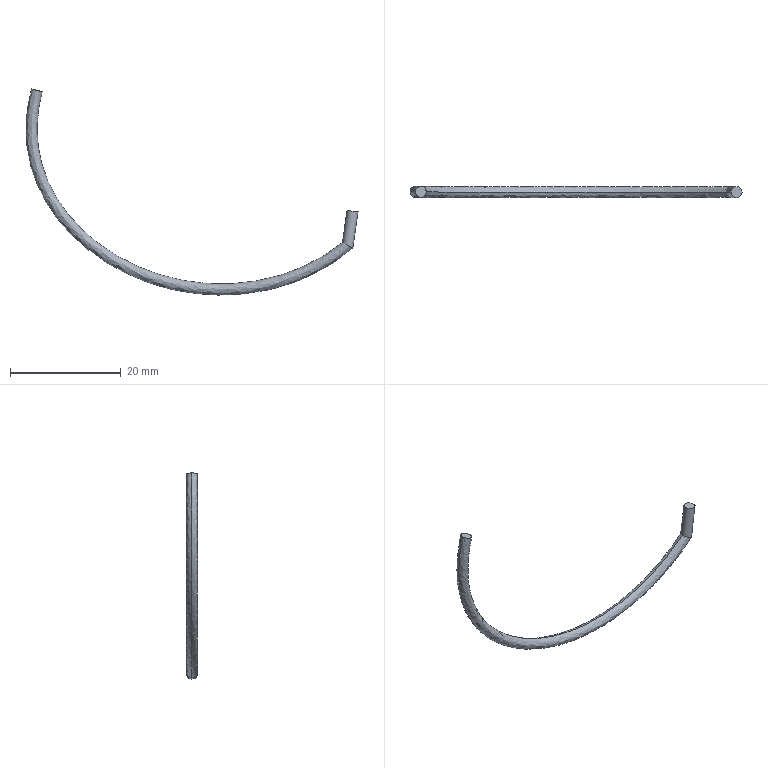Part | STEP file | YINGXIAN2_15_1 | 1 solid | 6 faces | box 59.863 x 2 x 37.179 mm | volume 274.797 mm3 | plane 2 | cylinder 2 | spline 2 | commonest cylinder face diameters 2 x2
STEP:
#1=CARTESIAN_POINT('',(0.,0.,0.));
#2=DIRECTION('',(0.,0.,1.));
#3=DIRECTION('',(1.,0.,0.));
#4=AXIS2_PLACEMENT_3D('',#1,#2,#3);
#5=CARTESIAN_POINT('',(50.419,0.,13.842));
#6=VERTEX_POINT('',#5);
#7=CARTESIAN_POINT('',(52.399,0.,13.558));
#8=VERTEX_POINT('',#7);
#9=CARTESIAN_POINT('',(51.409,0.,13.7));
#10=DIRECTION('',(-0.1418,0.,-0.9899));
#11=DIRECTION('',(-0.9899,0.,0.1418));
#12=AXIS2_PLACEMENT_3D('',#9,#10,#11);
#13=CIRCLE('',#12,1.);
#14=EDGE_CURVE('',#6,#8,#13,.T.);
#15=ORIENTED_EDGE('',*,*,#14,.T.);
#16=CARTESIAN_POINT('',(51.409,0.,13.7));
#17=DIRECTION('',(-0.1418,0.,-0.9899));
#18=DIRECTION('',(0.9899,0.,-0.1418));
#19=AXIS2_PLACEMENT_3D('',#16,#17,#18);
#20=CIRCLE('',#19,1.);
#21=EDGE_CURVE('',#8,#6,#20,.T.);
#22=ORIENTED_EDGE('',*,*,#21,.T.);
#23=EDGE_LOOP('',(#15,#22));
#24=FACE_OUTER_BOUND('',#23,.F.);
#25=CARTESIAN_POINT('',(51.409,0.,13.7));
#26=DIRECTION('',(-0.1418,0.,-0.9899));
#27=DIRECTION('',(-0.9899,0.,0.1418));
#28=AXIS2_PLACEMENT_3D('',#25,#26,#27);
#29=PLANE('',#28);
#30=ADVANCED_FACE('',(#24),#29,.F.);
#31=ORIENTED_EDGE('',*,*,#14,.F.);
#32=CARTESIAN_POINT('',(49.595,0.,8.085));
#33=VERTEX_POINT('',#32);
#34=CARTESIAN_POINT('',(50.419,0.,13.842));
#35=DIRECTION('',(-0.1418,0.,-0.9899));
#36=VECTOR('',#35,5.815);
#37=LINE('',#34,#36);
#38=EDGE_CURVE('',#6,#33,#37,.T.);
#39=ORIENTED_EDGE('',*,*,#38,.T.);
#40=CARTESIAN_POINT('',(50.53,1.,7.56));
#41=VERTEX_POINT('',#40);
#42=CARTESIAN_POINT('',(49.595,0.,8.085));
#43=CARTESIAN_POINT('',(49.595,0.08219,8.085));
#44=CARTESIAN_POINT('',(49.613,0.2494,8.076));
#45=CARTESIAN_POINT('',(49.713,0.5091,8.019));
#46=CARTESIAN_POINT('',(49.85,0.7019,7.942));
#47=CARTESIAN_POINT('',(50.052,0.873,7.828));
#48=CARTESIAN_POINT('',(50.269,0.9721,7.704));
#49=CARTESIAN_POINT('',(50.443,1.,7.611));
#50=B_SPLINE_CURVE_WITH_KNOTS('',3,(#42,#43,#44,#45,#46,#47,#48,#49,#40),.UNSPECIFIED.,.F.,.F.,(4,1,1,1,1,1,4),(0.,0.1667,0.3333,0.5,0.6667,0.8333,1.),.UNSPECIFIED.);
#51=EDGE_CURVE('',#33,#41,#50,.T.);
#52=ORIENTED_EDGE('',*,*,#51,.T.);
#53=CARTESIAN_POINT('',(51.466,0.,7.041));
#54=VERTEX_POINT('',#53);
#55=CARTESIAN_POINT('',(50.53,1.,7.56));
#56=CARTESIAN_POINT('',(50.615,1.,7.51));
#57=CARTESIAN_POINT('',(50.785,0.9732,7.419));
#58=CARTESIAN_POINT('',(50.998,0.8796,7.299));
#59=CARTESIAN_POINT('',(51.21,0.7043,7.182));
#60=CARTESIAN_POINT('',(51.351,0.5023,7.104));
#61=CARTESIAN_POINT('',(51.449,0.2456,7.051));
#62=CARTESIAN_POINT('',(51.466,0.0805,7.041));
#63=B_SPLINE_CURVE_WITH_KNOTS('',3,(#55,#56,#57,#58,#59,#60,#61,#62,#53),.UNSPECIFIED.,.F.,.F.,(4,1,1,1,1,1,4),(0.,0.1667,0.3333,0.5,0.6667,0.8333,1.),.UNSPECIFIED.);
#64=EDGE_CURVE('',#41,#54,#63,.T.);
#65=ORIENTED_EDGE('',*,*,#64,.T.);
#66=CARTESIAN_POINT('',(52.399,0.,13.558));
#67=DIRECTION('',(-0.1418,0.,-0.9899));
#68=VECTOR('',#67,6.584);
#69=LINE('',#66,#68);
#70=EDGE_CURVE('',#8,#54,#69,.T.);
#71=ORIENTED_EDGE('',*,*,#70,.F.);
#72=EDGE_LOOP('',(#31,#39,#52,#65,#71));
#73=FACE_OUTER_BOUND('',#72,.F.);
#74=CARTESIAN_POINT('',(51.409,0.,13.7));
#75=DIRECTION('',(-0.1418,0.,-0.9899));
#76=DIRECTION('',(-0.9899,0.,0.1418));
#77=AXIS2_PLACEMENT_3D('',#74,#75,#76);
#78=CYLINDRICAL_SURFACE('',#77,1.);
#79=ADVANCED_FACE('',(#73),#78,.T.);
#80=ORIENTED_EDGE('',*,*,#21,.F.);
#81=ORIENTED_EDGE('',*,*,#70,.T.);
#82=CARTESIAN_POINT('',(50.53,-1.,7.56));
#83=VERTEX_POINT('',#82);
#84=CARTESIAN_POINT('',(51.466,0.,7.041));
#85=CARTESIAN_POINT('',(51.466,-0.0826,7.041));
#86=CARTESIAN_POINT('',(51.448,-0.2503,7.051));
#87=CARTESIAN_POINT('',(51.348,-0.5086,7.106));
#88=CARTESIAN_POINT('',(51.211,-0.7022,7.182));
#89=CARTESIAN_POINT('',(51.008,-0.8734,7.294));
#90=CARTESIAN_POINT('',(50.79,-0.9723,7.416));
#91=CARTESIAN_POINT('',(50.617,-1.,7.509));
#92=B_SPLINE_CURVE_WITH_KNOTS('',3,(#84,#85,#86,#87,#88,#89,#90,#91,#82),.UNSPECIFIED.,.F.,.F.,(4,1,1,1,1,1,4),(0.,0.1667,0.3333,0.5,0.6667,0.8333,1.),.UNSPECIFIED.);
#93=EDGE_CURVE('',#54,#83,#92,.T.);
#94=ORIENTED_EDGE('',*,*,#93,.T.);
#95=CARTESIAN_POINT('',(50.53,-1.,7.56));
#96=CARTESIAN_POINT('',(50.445,-1.,7.61));
#97=CARTESIAN_POINT('',(50.274,-0.9729,7.702));
#98=CARTESIAN_POINT('',(50.061,-0.879,7.823));
#99=CARTESIAN_POINT('',(49.85,-0.7034,7.942));
#100=CARTESIAN_POINT('',(49.709,-0.5023,8.021));
#101=CARTESIAN_POINT('',(49.612,-0.2439,8.076));
#102=CARTESIAN_POINT('',(49.595,-0.07979,8.085));
#103=CARTESIAN_POINT('',(49.595,0.,8.085));
#104=B_SPLINE_CURVE_WITH_KNOTS('',3,(#95,#96,#97,#98,#99,#100,#101,#102,#103),.UNSPECIFIED.,.F.,.F.,(4,1,1,1,1,1,4),(0.,0.1667,0.3333,0.5,0.6667,0.8333,1.),.UNSPECIFIED.);
#105=EDGE_CURVE('',#83,#33,#104,.T.);
#106=ORIENTED_EDGE('',*,*,#105,.T.);
#107=ORIENTED_EDGE('',*,*,#38,.F.);
#108=EDGE_LOOP('',(#80,#81,#94,#106,#107));
#109=FACE_OUTER_BOUND('',#108,.F.);
#110=CARTESIAN_POINT('',(51.409,0.,13.7));
#111=DIRECTION('',(-0.1418,0.,-0.9899));
#112=DIRECTION('',(-0.9899,0.,0.1418));
#113=AXIS2_PLACEMENT_3D('',#110,#111,#112);
#114=CYLINDRICAL_SURFACE('',#113,1.);
#115=ADVANCED_FACE('',(#109),#114,.T.);
#116=ORIENTED_EDGE('',*,*,#93,.F.);
#117=CARTESIAN_POINT('',(-6.476,0.,35.75));
#118=VERTEX_POINT('',#117);
#119=CARTESIAN_POINT('',(51.466,0.,7.041));
#120=CARTESIAN_POINT('',(51.368,0.,6.957));
#121=CARTESIAN_POINT('',(48.473,0.,4.516));
#122=CARTESIAN_POINT('',(43.598,0.,1.651));
#123=CARTESIAN_POINT('',(36.447,0.,-0.6002));
#124=CARTESIAN_POINT('',(30.891,0.,-1.438));
#125=CARTESIAN_POINT('',(25.282,0.,-1.472));
#126=CARTESIAN_POINT('',(19.88,0.,-0.7714));
#127=CARTESIAN_POINT('',(14.311,0.,0.7748));
#128=CARTESIAN_POINT('',(9.081,0.,3.12));
#129=CARTESIAN_POINT('',(4.225,0.,6.241));
#130=CARTESIAN_POINT('',(-1.55,0.,11.378));
#131=CARTESIAN_POINT('',(-6.039,0.,18.405));
#132=CARTESIAN_POINT('',(-7.838,0.,27.383));
#133=CARTESIAN_POINT('',(-7.264,0.,32.827));
#134=B_SPLINE_CURVE_WITH_KNOTS('',3,(#119,#120,#121,#122,#123,#124,#125,#126,#127,#128,#129,#130,#131,#132,#133,#117),.UNSPECIFIED.,.F.,.F.,(4,1,1,1,1,1,1,1,1,1,1,1,1,4),(0.,0.004598,0.1351,0.2029,0.2764,0.3381,0.4048,0.4716,0.5439,0.6078,0.6771,0.8213,0.9071,1.),.UNSPECIFIED.);
#135=EDGE_CURVE('',#54,#118,#134,.T.);
#136=ORIENTED_EDGE('',*,*,#135,.T.);
#137=CARTESIAN_POINT('',(-4.544,0.,35.23));
#138=VERTEX_POINT('',#137);
#139=CARTESIAN_POINT('',(-4.544,-0.1199,35.23));
#140=CARTESIAN_POINT('',(-4.587,-0.3782,35.241));
#141=CARTESIAN_POINT('',(-4.813,-0.7341,35.302));
#142=CARTESIAN_POINT('',(-5.098,-0.9213,35.379));
#143=CARTESIAN_POINT('',(-5.338,-0.9899,35.444));
#144=CARTESIAN_POINT('',(-5.51,-1.005,35.49));
#145=CARTESIAN_POINT('',(-5.682,-0.9899,35.536));
#146=CARTESIAN_POINT('',(-5.922,-0.9213,35.601));
#147=CARTESIAN_POINT('',(-6.207,-0.7341,35.678));
#148=CARTESIAN_POINT('',(-6.433,-0.3782,35.739));
#149=CARTESIAN_POINT('',(-6.476,-0.1199,35.75));
#150=CARTESIAN_POINT('',(-6.476,0.,35.75));
#151=B_SPLINE_CURVE_WITH_KNOTS('',3,(#137,#139,#140,#141,#142,#143,#144,#145,#146,#147,#148,#149,#150),.UNSPECIFIED.,.F.,.F.,(4,1,1,1,1,1,1,1,1,1,4),(0.,0.125,0.25,0.375,0.4375,0.5,0.5625,0.625,0.75,0.875,1.),.UNSPECIFIED.);
#152=EDGE_CURVE('',#138,#118,#151,.T.);
#153=ORIENTED_EDGE('',*,*,#152,.F.);
#154=CARTESIAN_POINT('',(49.595,0.,8.085));
#155=CARTESIAN_POINT('',(47.029,0.,5.998));
#156=CARTESIAN_POINT('',(42.64,0.,3.449));
#157=CARTESIAN_POINT('',(35.999,0.,1.357));
#158=CARTESIAN_POINT('',(30.732,0.,0.5625));
#159=CARTESIAN_POINT('',(25.408,0.,0.5302));
#160=CARTESIAN_POINT('',(20.278,0.,1.196));
#161=CARTESIAN_POINT('',(14.995,0.,2.662));
#162=CARTESIAN_POINT('',(10.032,0.,4.887));
#163=CARTESIAN_POINT('',(5.436,0.,7.842));
#164=CARTESIAN_POINT('',(0.0008732,0.,12.681));
#165=CARTESIAN_POINT('',(-4.156,0.,19.212));
#166=CARTESIAN_POINT('',(-5.806,0.,27.461));
#167=CARTESIAN_POINT('',(-5.281,0.,32.497));
#168=CARTESIAN_POINT('',(-4.544,0.,35.23));
#169=B_SPLINE_CURVE_WITH_KNOTS('',3,(#154,#155,#156,#157,#158,#159,#160,#161,#162,#163,#164,#165,#166,#167,#168),.UNSPECIFIED.,.F.,.F.,(4,1,1,1,1,1,1,1,1,1,1,1,4),(0.,0.1269,0.1954,0.2696,0.3318,0.3992,0.4666,0.5396,0.6041,0.674,0.8196,0.9062,1.),.UNSPECIFIED.);
#170=EDGE_CURVE('',#33,#138,#169,.T.);
#171=ORIENTED_EDGE('',*,*,#170,.F.);
#172=ORIENTED_EDGE('',*,*,#105,.F.);
#173=EDGE_LOOP('',(#116,#136,#153,#171,#172));
#174=FACE_OUTER_BOUND('',#173,.F.);
#175=CARTESIAN_POINT('',(52.097,0.04715,7.595));
#176=CARTESIAN_POINT('',(51.792,0.04715,7.321));
#177=CARTESIAN_POINT('',(48.712,0.04715,4.658));
#178=CARTESIAN_POINT('',(43.598,0.04715,1.652));
#179=CARTESIAN_POINT('',(36.447,0.04715,-0.5991));
#180=CARTESIAN_POINT('',(30.891,0.04715,-1.437));
#181=CARTESIAN_POINT('',(25.282,0.04715,-1.471));
#182=CARTESIAN_POINT('',(19.88,0.04715,-0.7702));
#183=CARTESIAN_POINT('',(14.312,0.04715,0.7759));
#184=CARTESIAN_POINT('',(9.082,0.04715,3.121));
#185=CARTESIAN_POINT('',(4.225,0.04715,6.242));
#186=CARTESIAN_POINT('',(-1.549,0.04715,11.379));
#187=CARTESIAN_POINT('',(-6.038,0.04715,18.406));
#188=CARTESIAN_POINT('',(-7.884,0.04715,27.621));
#189=CARTESIAN_POINT('',(-7.204,0.04715,33.35));
#190=CARTESIAN_POINT('',(-6.244,0.04715,36.561));
#191=CARTESIAN_POINT('',(52.101,-0.08562,7.59));
#192=CARTESIAN_POINT('',(51.796,-0.08562,7.316));
#193=CARTESIAN_POINT('',(48.715,-0.08562,4.652));
#194=CARTESIAN_POINT('',(43.6,-0.08562,1.646));
#195=CARTESIAN_POINT('',(36.448,-0.08562,-0.6055));
#196=CARTESIAN_POINT('',(30.891,-0.08562,-1.444));
#197=CARTESIAN_POINT('',(25.282,-0.08562,-1.477));
#198=CARTESIAN_POINT('',(19.879,-0.08562,-0.7766));
#199=CARTESIAN_POINT('',(14.309,-0.08562,0.7697));
#200=CARTESIAN_POINT('',(9.078,-0.08562,3.115));
#201=CARTESIAN_POINT('',(4.221,-0.08562,6.237));
#202=CARTESIAN_POINT('',(-1.554,-0.08562,11.375));
#203=CARTESIAN_POINT('',(-6.044,-0.08562,18.403));
#204=CARTESIAN_POINT('',(-7.891,-0.08562,27.621));
#205=CARTESIAN_POINT('',(-7.21,-0.08563,33.351));
#206=CARTESIAN_POINT('',(-6.25,-0.08562,36.563));
#207=CARTESIAN_POINT('',(52.075,-0.3625,7.619));
#208=CARTESIAN_POINT('',(51.77,-0.3625,7.346));
#209=CARTESIAN_POINT('',(48.693,-0.3625,4.685));
#210=CARTESIAN_POINT('',(43.584,-0.3625,1.682));
#211=CARTESIAN_POINT('',(36.439,-0.3625,-0.5669));
#212=CARTESIAN_POINT('',(30.888,-0.3625,-1.404));
#213=CARTESIAN_POINT('',(25.284,-0.3625,-1.438));
#214=CARTESIAN_POINT('',(19.887,-0.3625,-0.7379));
#215=CARTESIAN_POINT('',(14.323,-0.3625,0.8069));
#216=CARTESIAN_POINT('',(9.097,-0.3625,3.15));
#217=CARTESIAN_POINT('',(4.245,-0.3625,6.268));
#218=CARTESIAN_POINT('',(-1.524,-0.3625,11.401));
#219=CARTESIAN_POINT('',(-6.007,-0.3625,18.419));
#220=CARTESIAN_POINT('',(-7.851,-0.3625,27.622));
#221=CARTESIAN_POINT('',(-7.171,-0.3625,33.344));
#222=CARTESIAN_POINT('',(-6.212,-0.3625,36.552));
#223=CARTESIAN_POINT('',(51.912,-0.7341,7.801));
#224=CARTESIAN_POINT('',(51.61,-0.7341,7.529));
#225=CARTESIAN_POINT('',(48.555,-0.7341,4.888));
#226=CARTESIAN_POINT('',(43.482,-0.7341,1.906));
#227=CARTESIAN_POINT('',(36.385,-0.7341,-0.3283));
#228=CARTESIAN_POINT('',(30.869,-0.7341,-1.16));
#229=CARTESIAN_POINT('',(25.3,-0.7341,-1.194));
#230=CARTESIAN_POINT('',(19.935,-0.7341,-0.4981));
#231=CARTESIAN_POINT('',(14.406,-0.7341,1.037));
#232=CARTESIAN_POINT('',(9.213,-0.7341,3.365));
#233=CARTESIAN_POINT('',(4.393,-0.7341,6.464));
#234=CARTESIAN_POINT('',(-1.335,-0.7341,11.559));
#235=CARTESIAN_POINT('',(-5.778,-0.7341,18.517));
#236=CARTESIAN_POINT('',(-7.603,-0.7341,27.629));
#237=CARTESIAN_POINT('',(-6.93,-0.7341,33.299));
#238=CARTESIAN_POINT('',(-5.979,-0.7341,36.482));
#239=CARTESIAN_POINT('',(51.715,-0.9213,8.021));
#240=CARTESIAN_POINT('',(51.415,-0.9213,7.752));
#241=CARTESIAN_POINT('',(48.387,-0.9213,5.134));
#242=CARTESIAN_POINT('',(43.358,-0.9213,2.178));
#243=CARTESIAN_POINT('',(36.318,-0.9213,-0.03895));
#244=CARTESIAN_POINT('',(30.845,-0.9213,-0.8645));
#245=CARTESIAN_POINT('',(25.318,-0.9213,-0.8978));
#246=CARTESIAN_POINT('',(19.994,-0.9213,-0.2073));
#247=CARTESIAN_POINT('',(14.507,-0.9213,1.316));
#248=CARTESIAN_POINT('',(9.354,-0.9213,3.626));
#249=CARTESIAN_POINT('',(4.572,-0.9213,6.7));
#250=CARTESIAN_POINT('',(-1.105,-0.9213,11.752));
#251=CARTESIAN_POINT('',(-5.499,-0.9213,18.637));
#252=CARTESIAN_POINT('',(-7.302,-0.9213,27.638));
#253=CARTESIAN_POINT('',(-6.638,-0.9214,33.244));
#254=CARTESIAN_POINT('',(-5.695,-0.9213,36.397));
#255=CARTESIAN_POINT('',(51.549,-0.9898,8.206));
#256=CARTESIAN_POINT('',(51.251,-0.9898,7.939));
#257=CARTESIAN_POINT('',(48.245,-0.9899,5.34));
#258=CARTESIAN_POINT('',(43.254,-0.9899,2.406));
#259=CARTESIAN_POINT('',(36.262,-0.9899,0.2046));
#260=CARTESIAN_POINT('',(30.825,-0.9899,-0.6155));
#261=CARTESIAN_POINT('',(25.334,-0.9899,-0.6486));
#262=CARTESIAN_POINT('',(20.044,-0.9899,0.03745));
#263=CARTESIAN_POINT('',(14.592,-0.9898,1.551));
#264=CARTESIAN_POINT('',(9.472,-0.9899,3.846));
#265=CARTESIAN_POINT('',(4.723,-0.9899,6.9));
#266=CARTESIAN_POINT('',(-0.9124,-0.9899,11.914));
#267=CARTESIAN_POINT('',(-5.265,-0.9899,18.737));
#268=CARTESIAN_POINT('',(-7.048,-0.9898,27.645));
#269=CARTESIAN_POINT('',(-6.392,-0.9899,33.198));
#270=CARTESIAN_POINT('',(-5.457,-0.9898,36.326));
#271=CARTESIAN_POINT('',(51.43,-1.005,8.338));
#272=CARTESIAN_POINT('',(51.134,-1.005,8.073));
#273=CARTESIAN_POINT('',(48.145,-1.005,5.488));
#274=CARTESIAN_POINT('',(43.179,-1.005,2.569));
#275=CARTESIAN_POINT('',(36.223,-1.005,0.3785));
#276=CARTESIAN_POINT('',(30.811,-1.005,-0.4378));
#277=CARTESIAN_POINT('',(25.345,-1.005,-0.4708));
#278=CARTESIAN_POINT('',(20.079,-1.005,0.2121));
#279=CARTESIAN_POINT('',(14.653,-1.005,1.719));
#280=CARTESIAN_POINT('',(9.557,-1.005,4.003));
#281=CARTESIAN_POINT('',(4.831,-1.005,7.042));
#282=CARTESIAN_POINT('',(-0.7747,-1.005,12.03));
#283=CARTESIAN_POINT('',(-5.097,-1.005,18.809));
#284=CARTESIAN_POINT('',(-6.868,-1.005,27.65));
#285=CARTESIAN_POINT('',(-6.216,-1.005,33.165));
#286=CARTESIAN_POINT('',(-5.287,-1.005,36.275));
#287=CARTESIAN_POINT('',(51.311,-0.9898,8.471));
#288=CARTESIAN_POINT('',(51.017,-0.9898,8.207));
#289=CARTESIAN_POINT('',(48.044,-0.9899,5.636));
#290=CARTESIAN_POINT('',(43.105,-0.9899,2.732));
#291=CARTESIAN_POINT('',(36.183,-0.9899,0.5523));
#292=CARTESIAN_POINT('',(30.797,-0.9899,-0.2602));
#293=CARTESIAN_POINT('',(25.356,-0.9899,-0.293));
#294=CARTESIAN_POINT('',(20.114,-0.9899,0.3868));
#295=CARTESIAN_POINT('',(14.714,-0.9898,1.886));
#296=CARTESIAN_POINT('',(9.641,-0.9899,4.16));
#297=CARTESIAN_POINT('',(4.938,-0.9899,7.184));
#298=CARTESIAN_POINT('',(-0.6369,-0.9899,12.145));
#299=CARTESIAN_POINT('',(-4.93,-0.9899,18.88));
#300=CARTESIAN_POINT('',(-6.687,-0.9898,27.655));
#301=CARTESIAN_POINT('',(-6.041,-0.9899,33.133));
#302=CARTESIAN_POINT('',(-5.117,-0.9898,36.224));
#303=CARTESIAN_POINT('',(51.145,-0.9213,8.656));
#304=CARTESIAN_POINT('',(50.853,-0.9213,8.394));
#305=CARTESIAN_POINT('',(47.903,-0.9213,5.843));
#306=CARTESIAN_POINT('',(43.001,-0.9213,2.961));
#307=CARTESIAN_POINT('',(36.127,-0.9213,0.7959));
#308=CARTESIAN_POINT('',(30.777,-0.9213,-0.0112));
#309=CARTESIAN_POINT('',(25.372,-0.9213,-0.04387));
#310=CARTESIAN_POINT('',(20.164,-0.9213,0.6316));
#311=CARTESIAN_POINT('',(14.799,-0.9213,2.121));
#312=CARTESIAN_POINT('',(9.759,-0.9213,4.38));
#313=CARTESIAN_POINT('',(5.089,-0.9213,7.383));
#314=CARTESIAN_POINT('',(-0.4439,-0.9213,12.307));
#315=CARTESIAN_POINT('',(-4.696,-0.9213,18.981));
#316=CARTESIAN_POINT('',(-6.434,-0.9213,27.663));
#317=CARTESIAN_POINT('',(-5.795,-0.9214,33.087));
#318=CARTESIAN_POINT('',(-4.878,-0.9213,36.153));
#319=CARTESIAN_POINT('',(50.948,-0.7341,8.876));
#320=CARTESIAN_POINT('',(50.658,-0.7341,8.616));
#321=CARTESIAN_POINT('',(47.735,-0.7341,6.088));
#322=CARTESIAN_POINT('',(42.877,-0.7341,3.232));
#323=CARTESIAN_POINT('',(36.061,-0.7341,1.085));
#324=CARTESIAN_POINT('',(30.754,-0.7341,0.2845));
#325=CARTESIAN_POINT('',(25.39,-0.7341,0.2521));
#326=CARTESIAN_POINT('',(20.222,-0.7341,0.9224));
#327=CARTESIAN_POINT('',(14.9,-0.7341,2.4));
#328=CARTESIAN_POINT('',(9.9,-0.7341,4.642));
#329=CARTESIAN_POINT('',(5.268,-0.7341,7.62));
#330=CARTESIAN_POINT('',(-0.2146,-0.7341,12.5));
#331=CARTESIAN_POINT('',(-4.417,-0.7341,19.1));
#332=CARTESIAN_POINT('',(-6.133,-0.7341,27.671));
#333=CARTESIAN_POINT('',(-5.502,-0.7341,33.032));
#334=CARTESIAN_POINT('',(-4.595,-0.7341,36.068));
#335=CARTESIAN_POINT('',(50.785,-0.3629,9.057));
#336=CARTESIAN_POINT('',(50.498,-0.3629,8.8));
#337=CARTESIAN_POINT('',(47.597,-0.3629,6.291));
#338=CARTESIAN_POINT('',(42.775,-0.3629,3.455));
#339=CARTESIAN_POINT('',(36.006,-0.3629,1.324));
#340=CARTESIAN_POINT('',(30.734,-0.3629,0.5282));
#341=CARTESIAN_POINT('',(25.406,-0.3629,0.4959));
#342=CARTESIAN_POINT('',(20.271,-0.3629,1.162));
#343=CARTESIAN_POINT('',(14.983,-0.3629,2.63));
#344=CARTESIAN_POINT('',(10.016,-0.3629,4.857));
#345=CARTESIAN_POINT('',(5.416,-0.3629,7.815));
#346=CARTESIAN_POINT('',(-0.02568,-0.3629,12.659));
#347=CARTESIAN_POINT('',(-4.188,-0.3629,19.198));
#348=CARTESIAN_POINT('',(-5.885,-0.3629,27.678));
#349=CARTESIAN_POINT('',(-5.261,-0.3629,32.987));
#350=CARTESIAN_POINT('',(-4.362,-0.3629,35.998));
#351=CARTESIAN_POINT('',(50.759,-0.08642,9.087));
#352=CARTESIAN_POINT('',(50.472,-0.08642,8.829));
#353=CARTESIAN_POINT('',(47.574,-0.08642,6.324));
#354=CARTESIAN_POINT('',(42.758,-0.08642,3.492));
#355=CARTESIAN_POINT('',(35.997,-0.08642,1.362));
#356=CARTESIAN_POINT('',(30.731,-0.08642,0.5677));
#357=CARTESIAN_POINT('',(25.408,-0.08642,0.5355));
#358=CARTESIAN_POINT('',(20.279,-0.08642,1.201));
#359=CARTESIAN_POINT('',(14.996,-0.08642,2.667));
#360=CARTESIAN_POINT('',(10.035,-0.08642,4.892));
#361=CARTESIAN_POINT('',(5.44,-0.08642,7.847));
#362=CARTESIAN_POINT('',(0.004959,-0.08642,12.684));
#363=CARTESIAN_POINT('',(-4.151,-0.08642,19.214));
#364=CARTESIAN_POINT('',(-5.845,-0.08642,27.68));
#365=CARTESIAN_POINT('',(-5.222,-0.08643,32.98));
#366=CARTESIAN_POINT('',(-4.324,-0.08642,35.987));
#367=CARTESIAN_POINT('',(50.763,0.04607,9.082));
#368=CARTESIAN_POINT('',(50.476,0.04607,8.825));
#369=CARTESIAN_POINT('',(47.578,0.04607,6.319));
#370=CARTESIAN_POINT('',(42.761,0.04607,3.486));
#371=CARTESIAN_POINT('',(35.999,0.04607,1.356));
#372=CARTESIAN_POINT('',(30.732,0.04607,0.5614));
#373=CARTESIAN_POINT('',(25.408,0.04607,0.5291));
#374=CARTESIAN_POINT('',(20.277,0.04607,1.195));
#375=CARTESIAN_POINT('',(14.994,0.04607,2.661));
#376=CARTESIAN_POINT('',(10.032,0.04607,4.886));
#377=CARTESIAN_POINT('',(5.436,0.04607,7.841));
#378=CARTESIAN_POINT('',(0.00001944,0.04607,12.68));
#379=CARTESIAN_POINT('',(-4.157,0.04607,19.212));
#380=CARTESIAN_POINT('',(-5.851,0.04606,27.679));
#381=CARTESIAN_POINT('',(-5.229,0.04607,32.981));
#382=CARTESIAN_POINT('',(-4.33,0.04607,35.989));
#383=B_SPLINE_SURFACE_WITH_KNOTS('',3,3,((#175,#176,#177,#178,#179,#180,#181,#182,#183,#184,#185,#186,#187,#188,#189,#190),(#191,#192,#193,#194,#195,#196,#197,#198,#199,#200,#201,#202,#203,#204,#205,#206),(#207,#208,#209,#210,#211,#212,#213,#214,#215,#216,#217,#218,#219,#220,#221,#222),(#223,#224,#225,#226,#227,#228,#229,#230,#231,#232,#233,#234,#235,#236,#237,#238),(#239,#240,#241,#242,#243,#244,#245,#246,#247,#248,#249,#250,#251,#252,#253,#254),(#255,#256,#257,#258,#259,#260,#261,#262,#263,#264,#265,#266,#267,#268,#269,#270),(#271,#272,#273,#274,#275,#276,#277,#278,#279,#280,#281,#282,#283,#284,#285,#286),(#287,#288,#289,#290,#291,#292,#293,#294,#295,#296,#297,#298,#299,#300,#301,#302),(#303,#304,#305,#306,#307,#308,#309,#310,#311,#312,#313,#314,#315,#316,#317,#318),(#319,#320,#321,#322,#323,#324,#325,#326,#327,#328,#329,#330,#331,#332,#333,#334),(#335,#336,#337,#338,#339,#340,#341,#342,#343,#344,#345,#346,#347,#348,#349,#350),(#351,#352,#353,#354,#355,#356,#357,#358,#359,#360,#361,#362,#363,#364,#365,#366),(#367,#368,#369,#370,#371,#372,#373,#374,#375,#376,#377,#378,#379,#380,#381,#382)),.UNSPECIFIED.,.F.,.F.,.F.,(4,1,1,1,1,1,1,1,1,1,4),(4,1,1,1,1,1,1,1,1,1,1,1,1,4),(0.02517,0.2923,0.5282,0.7641,0.8821,1.,1.118,1.236,1.472,1.708,1.974),(-0.01463,0.,0.1311,0.1993,0.2731,0.335,0.4021,0.4692,0.5418,0.606,0.6756,0.8204,0.9066,1.009),.UNSPECIFIED.);
#384=ADVANCED_FACE('',(#174),#383,.T.);
#385=ORIENTED_EDGE('',*,*,#51,.F.);
#386=ORIENTED_EDGE('',*,*,#170,.T.);
#387=CARTESIAN_POINT('',(-6.476,0.,35.75));
#388=CARTESIAN_POINT('',(-6.476,0.1199,35.75));
#389=CARTESIAN_POINT('',(-6.433,0.3782,35.739));
#390=CARTESIAN_POINT('',(-6.207,0.7341,35.678));
#391=CARTESIAN_POINT('',(-5.922,0.9213,35.601));
#392=CARTESIAN_POINT('',(-5.682,0.9899,35.536));
#393=CARTESIAN_POINT('',(-5.51,1.005,35.49));
#394=CARTESIAN_POINT('',(-5.338,0.9899,35.444));
#395=CARTESIAN_POINT('',(-5.098,0.9213,35.379));
#396=CARTESIAN_POINT('',(-4.813,0.7341,35.302));
#397=CARTESIAN_POINT('',(-4.587,0.3782,35.241));
#398=CARTESIAN_POINT('',(-4.544,0.1199,35.23));
#399=CARTESIAN_POINT('',(-4.544,0.,35.23));
#400=B_SPLINE_CURVE_WITH_KNOTS('',3,(#387,#388,#389,#390,#391,#392,#393,#394,#395,#396,#397,#398,#399),.UNSPECIFIED.,.F.,.F.,(4,1,1,1,1,1,1,1,1,1,4),(0.,0.125,0.25,0.375,0.4375,0.5,0.5625,0.625,0.75,0.875,1.),.UNSPECIFIED.);
#401=EDGE_CURVE('',#118,#138,#400,.T.);
#402=ORIENTED_EDGE('',*,*,#401,.F.);
#403=ORIENTED_EDGE('',*,*,#135,.F.);
#404=ORIENTED_EDGE('',*,*,#64,.F.);
#405=EDGE_LOOP('',(#385,#386,#402,#403,#404));
#406=FACE_OUTER_BOUND('',#405,.F.);
#407=CARTESIAN_POINT('',(50.763,-0.04715,9.082));
#408=CARTESIAN_POINT('',(50.476,-0.04715,8.825));
#409=CARTESIAN_POINT('',(47.578,-0.04715,6.318));
#410=CARTESIAN_POINT('',(42.761,-0.04715,3.486));
#411=CARTESIAN_POINT('',(35.999,-0.04715,1.356));
#412=CARTESIAN_POINT('',(30.732,-0.04715,0.5613));
#413=CARTESIAN_POINT('',(25.408,-0.04715,0.5291));
#414=CARTESIAN_POINT('',(20.277,-0.04715,1.195));
#415=CARTESIAN_POINT('',(14.994,-0.04715,2.661));
#416=CARTESIAN_POINT('',(10.032,-0.04715,4.886));
#417=CARTESIAN_POINT('',(5.436,-0.04715,7.841));
#418=CARTESIAN_POINT('',(-0.0000215,-0.04715,12.68));
#419=CARTESIAN_POINT('',(-4.157,-0.04715,19.212));
#420=CARTESIAN_POINT('',(-5.851,-0.04715,27.679));
#421=CARTESIAN_POINT('',(-5.229,-0.04715,32.981));
#422=CARTESIAN_POINT('',(-4.33,-0.04715,35.989));
#423=CARTESIAN_POINT('',(50.759,0.08562,9.087));
#424=CARTESIAN_POINT('',(50.472,0.08562,8.829));
#425=CARTESIAN_POINT('',(47.574,0.08562,6.324));
#426=CARTESIAN_POINT('',(42.758,0.08562,3.492));
#427=CARTESIAN_POINT('',(35.997,0.08562,1.362));
#428=CARTESIAN_POINT('',(30.731,0.08562,0.5678));
#429=CARTESIAN_POINT('',(25.408,0.08562,0.5356));
#430=CARTESIAN_POINT('',(20.279,0.08562,1.201));
#431=CARTESIAN_POINT('',(14.997,0.08562,2.667));
#432=CARTESIAN_POINT('',(10.035,0.08562,4.892));
#433=CARTESIAN_POINT('',(5.44,0.08562,7.847));
#434=CARTESIAN_POINT('',(0.005048,0.08562,12.685));
#435=CARTESIAN_POINT('',(-4.15,0.08562,19.214));
#436=CARTESIAN_POINT('',(-5.845,0.08562,27.68));
#437=CARTESIAN_POINT('',(-5.222,0.08563,32.98));
#438=CARTESIAN_POINT('',(-4.324,0.08562,35.987));
#439=CARTESIAN_POINT('',(50.785,0.3625,9.057));
#440=CARTESIAN_POINT('',(50.498,0.3625,8.8));
#441=CARTESIAN_POINT('',(47.596,0.3625,6.291));
#442=CARTESIAN_POINT('',(42.775,0.3625,3.456));
#443=CARTESIAN_POINT('',(36.006,0.3625,1.324));
#444=CARTESIAN_POINT('',(30.734,0.3625,0.5284));
#445=CARTESIAN_POINT('',(25.406,0.3625,0.4962));
#446=CARTESIAN_POINT('',(20.271,0.3625,1.162));
#447=CARTESIAN_POINT('',(14.983,0.3625,2.63));
#448=CARTESIAN_POINT('',(10.016,0.3625,4.857));
#449=CARTESIAN_POINT('',(5.416,0.3625,7.815));
#450=CARTESIAN_POINT('',(-0.0255,0.3625,12.659));
#451=CARTESIAN_POINT('',(-4.188,0.3625,19.198));
#452=CARTESIAN_POINT('',(-5.885,0.3625,27.678));
#453=CARTESIAN_POINT('',(-5.261,0.3625,32.987));
#454=CARTESIAN_POINT('',(-4.361,0.3625,35.998));
#455=CARTESIAN_POINT('',(50.948,0.7341,8.876));
#456=CARTESIAN_POINT('',(50.658,0.7341,8.616));
#457=CARTESIAN_POINT('',(47.735,0.7341,6.088));
#458=CARTESIAN_POINT('',(42.877,0.7341,3.232));
#459=CARTESIAN_POINT('',(36.061,0.7341,1.085));
#460=CARTESIAN_POINT('',(30.754,0.7341,0.2845));
#461=CARTESIAN_POINT('',(25.39,0.7341,0.2521));
#462=CARTESIAN_POINT('',(20.222,0.7341,0.9224));
#463=CARTESIAN_POINT('',(14.9,0.7341,2.4));
#464=CARTESIAN_POINT('',(9.9,0.7341,4.642));
#465=CARTESIAN_POINT('',(5.268,0.7341,7.62));
#466=CARTESIAN_POINT('',(-0.2146,0.7341,12.5));
#467=CARTESIAN_POINT('',(-4.417,0.7341,19.1));
#468=CARTESIAN_POINT('',(-6.133,0.7341,27.671));
#469=CARTESIAN_POINT('',(-5.502,0.7341,33.032));
#470=CARTESIAN_POINT('',(-4.595,0.7341,36.068));
#471=CARTESIAN_POINT('',(51.145,0.9213,8.656));
#472=CARTESIAN_POINT('',(50.853,0.9213,8.394));
#473=CARTESIAN_POINT('',(47.903,0.9213,5.843));
#474=CARTESIAN_POINT('',(43.001,0.9213,2.961));
#475=CARTESIAN_POINT('',(36.127,0.9213,0.7959));
#476=CARTESIAN_POINT('',(30.777,0.9213,-0.0112));
#477=CARTESIAN_POINT('',(25.372,0.9213,-0.04387));
#478=CARTESIAN_POINT('',(20.164,0.9213,0.6316));
#479=CARTESIAN_POINT('',(14.799,0.9213,2.121));
#480=CARTESIAN_POINT('',(9.759,0.9213,4.38));
#481=CARTESIAN_POINT('',(5.089,0.9213,7.383));
#482=CARTESIAN_POINT('',(-0.4439,0.9213,12.307));
#483=CARTESIAN_POINT('',(-4.696,0.9213,18.981));
#484=CARTESIAN_POINT('',(-6.434,0.9213,27.663));
#485=CARTESIAN_POINT('',(-5.795,0.9214,33.087));
#486=CARTESIAN_POINT('',(-4.878,0.9213,36.153));
#487=CARTESIAN_POINT('',(51.311,0.9898,8.471));
#488=CARTESIAN_POINT('',(51.017,0.9898,8.207));
#489=CARTESIAN_POINT('',(48.044,0.9899,5.636));
#490=CARTESIAN_POINT('',(43.105,0.9899,2.732));
#491=CARTESIAN_POINT('',(36.183,0.9899,0.5523));
#492=CARTESIAN_POINT('',(30.797,0.9899,-0.2602));
#493=CARTESIAN_POINT('',(25.356,0.9899,-0.293));
#494=CARTESIAN_POINT('',(20.114,0.9899,0.3868));
#495=CARTESIAN_POINT('',(14.714,0.9898,1.886));
#496=CARTESIAN_POINT('',(9.641,0.9899,4.16));
#497=CARTESIAN_POINT('',(4.938,0.9899,7.184));
#498=CARTESIAN_POINT('',(-0.6369,0.9899,12.145));
#499=CARTESIAN_POINT('',(-4.93,0.9899,18.88));
#500=CARTESIAN_POINT('',(-6.687,0.9898,27.655));
#501=CARTESIAN_POINT('',(-6.041,0.9899,33.133));
#502=CARTESIAN_POINT('',(-5.117,0.9898,36.224));
#503=CARTESIAN_POINT('',(51.43,1.005,8.338));
#504=CARTESIAN_POINT('',(51.134,1.005,8.073));
#505=CARTESIAN_POINT('',(48.145,1.005,5.488));
#506=CARTESIAN_POINT('',(43.179,1.005,2.569));
#507=CARTESIAN_POINT('',(36.223,1.005,0.3785));
#508=CARTESIAN_POINT('',(30.811,1.005,-0.4378));
#509=CARTESIAN_POINT('',(25.345,1.005,-0.4708));
#510=CARTESIAN_POINT('',(20.079,1.005,0.2121));
#511=CARTESIAN_POINT('',(14.653,1.005,1.719));
#512=CARTESIAN_POINT('',(9.557,1.005,4.003));
#513=CARTESIAN_POINT('',(4.831,1.005,7.042));
#514=CARTESIAN_POINT('',(-0.7747,1.005,12.03));
#515=CARTESIAN_POINT('',(-5.097,1.005,18.809));
#516=CARTESIAN_POINT('',(-6.868,1.005,27.65));
#517=CARTESIAN_POINT('',(-6.216,1.005,33.165));
#518=CARTESIAN_POINT('',(-5.287,1.005,36.275));
#519=CARTESIAN_POINT('',(51.549,0.9898,8.206));
#520=CARTESIAN_POINT('',(51.251,0.9898,7.939));
#521=CARTESIAN_POINT('',(48.245,0.9899,5.34));
#522=CARTESIAN_POINT('',(43.254,0.9899,2.406));
#523=CARTESIAN_POINT('',(36.262,0.9899,0.2046));
#524=CARTESIAN_POINT('',(30.825,0.9899,-0.6155));
#525=CARTESIAN_POINT('',(25.334,0.9899,-0.6486));
#526=CARTESIAN_POINT('',(20.044,0.9899,0.03745));
#527=CARTESIAN_POINT('',(14.592,0.9898,1.551));
#528=CARTESIAN_POINT('',(9.472,0.9899,3.846));
#529=CARTESIAN_POINT('',(4.723,0.9899,6.9));
#530=CARTESIAN_POINT('',(-0.9124,0.9899,11.914));
#531=CARTESIAN_POINT('',(-5.265,0.9899,18.737));
#532=CARTESIAN_POINT('',(-7.048,0.9898,27.645));
#533=CARTESIAN_POINT('',(-6.392,0.9899,33.198));
#534=CARTESIAN_POINT('',(-5.457,0.9898,36.326));
#535=CARTESIAN_POINT('',(51.715,0.9213,8.021));
#536=CARTESIAN_POINT('',(51.415,0.9213,7.752));
#537=CARTESIAN_POINT('',(48.387,0.9213,5.134));
#538=CARTESIAN_POINT('',(43.358,0.9213,2.178));
#539=CARTESIAN_POINT('',(36.318,0.9213,-0.03895));
#540=CARTESIAN_POINT('',(30.845,0.9213,-0.8645));
#541=CARTESIAN_POINT('',(25.318,0.9213,-0.8978));
#542=CARTESIAN_POINT('',(19.994,0.9213,-0.2073));
#543=CARTESIAN_POINT('',(14.507,0.9213,1.316));
#544=CARTESIAN_POINT('',(9.354,0.9213,3.626));
#545=CARTESIAN_POINT('',(4.572,0.9213,6.7));
#546=CARTESIAN_POINT('',(-1.105,0.9213,11.752));
#547=CARTESIAN_POINT('',(-5.499,0.9213,18.637));
#548=CARTESIAN_POINT('',(-7.302,0.9213,27.638));
#549=CARTESIAN_POINT('',(-6.638,0.9214,33.244));
#550=CARTESIAN_POINT('',(-5.695,0.9213,36.397));
#551=CARTESIAN_POINT('',(51.912,0.7341,7.801));
#552=CARTESIAN_POINT('',(51.61,0.7341,7.529));
#553=CARTESIAN_POINT('',(48.555,0.7341,4.888));
#554=CARTESIAN_POINT('',(43.482,0.7341,1.906));
#555=CARTESIAN_POINT('',(36.385,0.7341,-0.3283));
#556=CARTESIAN_POINT('',(30.869,0.7341,-1.16));
#557=CARTESIAN_POINT('',(25.3,0.7341,-1.194));
#558=CARTESIAN_POINT('',(19.935,0.7341,-0.4981));
#559=CARTESIAN_POINT('',(14.406,0.7341,1.037));
#560=CARTESIAN_POINT('',(9.213,0.7341,3.365));
#561=CARTESIAN_POINT('',(4.393,0.7341,6.464));
#562=CARTESIAN_POINT('',(-1.335,0.7341,11.559));
#563=CARTESIAN_POINT('',(-5.778,0.7341,18.517));
#564=CARTESIAN_POINT('',(-7.603,0.7341,27.629));
#565=CARTESIAN_POINT('',(-6.93,0.7341,33.299));
#566=CARTESIAN_POINT('',(-5.979,0.7341,36.482));
#567=CARTESIAN_POINT('',(52.075,0.3629,7.619));
#568=CARTESIAN_POINT('',(51.77,0.3629,7.346));
#569=CARTESIAN_POINT('',(48.693,0.3629,4.685));
#570=CARTESIAN_POINT('',(43.584,0.3629,1.683));
#571=CARTESIAN_POINT('',(36.439,0.3629,-0.5667));
#572=CARTESIAN_POINT('',(30.888,0.3629,-1.404));
#573=CARTESIAN_POINT('',(25.285,0.3629,-1.438));
#574=CARTESIAN_POINT('',(19.887,0.3629,-0.7377));
#575=CARTESIAN_POINT('',(14.323,0.3629,0.8071));
#576=CARTESIAN_POINT('',(9.097,0.3629,3.15));
#577=CARTESIAN_POINT('',(4.245,0.3629,6.269));
#578=CARTESIAN_POINT('',(-1.524,0.3629,11.401));
#579=CARTESIAN_POINT('',(-6.007,0.3629,18.419));
#580=CARTESIAN_POINT('',(-7.85,0.3629,27.622));
#581=CARTESIAN_POINT('',(-7.171,0.3629,33.344));
#582=CARTESIAN_POINT('',(-6.212,0.3629,36.552));
#583=CARTESIAN_POINT('',(52.101,0.08642,7.59));
#584=CARTESIAN_POINT('',(51.796,0.08642,7.316));
#585=CARTESIAN_POINT('',(48.715,0.08642,4.652));
#586=CARTESIAN_POINT('',(43.6,0.08642,1.646));
#587=CARTESIAN_POINT('',(36.448,0.08642,-0.6054));
#588=CARTESIAN_POINT('',(30.891,0.08642,-1.443));
#589=CARTESIAN_POINT('',(25.282,0.08642,-1.477));
#590=CARTESIAN_POINT('',(19.879,0.08642,-0.7765));
#591=CARTESIAN_POINT('',(14.309,0.08642,0.7698));
#592=CARTESIAN_POINT('',(9.079,0.08642,3.115));
#593=CARTESIAN_POINT('',(4.222,0.08642,6.237));
#594=CARTESIAN_POINT('',(-1.554,0.08642,11.375));
#595=CARTESIAN_POINT('',(-6.044,0.08642,18.403));
#596=CARTESIAN_POINT('',(-7.891,0.08642,27.621));
#597=CARTESIAN_POINT('',(-7.21,0.08643,33.351));
#598=CARTESIAN_POINT('',(-6.25,0.08642,36.563));
#599=CARTESIAN_POINT('',(52.097,-0.04607,7.595));
#600=CARTESIAN_POINT('',(51.792,-0.04607,7.321));
#601=CARTESIAN_POINT('',(48.712,-0.04607,4.658));
#602=CARTESIAN_POINT('',(43.598,-0.04607,1.652));
#603=CARTESIAN_POINT('',(36.447,-0.04607,-0.5991));
#604=CARTESIAN_POINT('',(30.891,-0.04607,-1.437));
#605=CARTESIAN_POINT('',(25.282,-0.04607,-1.471));
#606=CARTESIAN_POINT('',(19.88,-0.04607,-0.7703));
#607=CARTESIAN_POINT('',(14.312,-0.04607,0.7758));
#608=CARTESIAN_POINT('',(9.082,-0.04607,3.12));
#609=CARTESIAN_POINT('',(4.225,-0.04607,6.242));
#610=CARTESIAN_POINT('',(-1.549,-0.04607,11.379));
#611=CARTESIAN_POINT('',(-6.038,-0.04607,18.406));
#612=CARTESIAN_POINT('',(-7.884,-0.04606,27.621));
#613=CARTESIAN_POINT('',(-7.204,-0.04607,33.35));
#614=CARTESIAN_POINT('',(-6.244,-0.04607,36.561));
#615=B_SPLINE_SURFACE_WITH_KNOTS('',3,3,((#407,#408,#409,#410,#411,#412,#413,#414,#415,#416,#417,#418,#419,#420,#421,#422),(#423,#424,#425,#426,#427,#428,#429,#430,#431,#432,#433,#434,#435,#436,#437,#438),(#439,#440,#441,#442,#443,#444,#445,#446,#447,#448,#449,#450,#451,#452,#453,#454),(#455,#456,#457,#458,#459,#460,#461,#462,#463,#464,#465,#466,#467,#468,#469,#470),(#471,#472,#473,#474,#475,#476,#477,#478,#479,#480,#481,#482,#483,#484,#485,#486),(#487,#488,#489,#490,#491,#492,#493,#494,#495,#496,#497,#498,#499,#500,#501,#502),(#503,#504,#505,#506,#507,#508,#509,#510,#511,#512,#513,#514,#515,#516,#517,#518),(#519,#520,#521,#522,#523,#524,#525,#526,#527,#528,#529,#530,#531,#532,#533,#534),(#535,#536,#537,#538,#539,#540,#541,#542,#543,#544,#545,#546,#547,#548,#549,#550),(#551,#552,#553,#554,#555,#556,#557,#558,#559,#560,#561,#562,#563,#564,#565,#566),(#567,#568,#569,#570,#571,#572,#573,#574,#575,#576,#577,#578,#579,#580,#581,#582),(#583,#584,#585,#586,#587,#588,#589,#590,#591,#592,#593,#594,#595,#596,#597,#598),(#599,#600,#601,#602,#603,#604,#605,#606,#607,#608,#609,#610,#611,#612,#613,#614)),.UNSPECIFIED.,.F.,.F.,.F.,(4,1,1,1,1,1,1,1,1,1,4),(4,1,1,1,1,1,1,1,1,1,1,1,1,4),(0.02517,0.2923,0.5282,0.7641,0.8821,1.,1.118,1.236,1.472,1.708,1.974),(-0.01463,0.,0.1311,0.1993,0.2731,0.335,0.4021,0.4692,0.5418,0.606,0.6756,0.8204,0.9066,1.009),.UNSPECIFIED.);
#616=ADVANCED_FACE('',(#406),#615,.T.);
#617=ORIENTED_EDGE('',*,*,#401,.T.);
#618=ORIENTED_EDGE('',*,*,#152,.T.);
#619=EDGE_LOOP('',(#617,#618));
#620=FACE_OUTER_BOUND('',#619,.F.);
#621=CARTESIAN_POINT('',(-5.51,0.,35.49));
#622=DIRECTION('',(0.2603,0.,0.9655));
#623=DIRECTION('',(0.9655,0.,-0.2603));
#624=AXIS2_PLACEMENT_3D('',#621,#622,#623);
#625=PLANE('',#624);
#626=ADVANCED_FACE('',(#620),#625,.T.);
#627=CLOSED_SHELL('',(#30,#79,#115,#384,#616,#626));
#628=MANIFOLD_SOLID_BREP('',#627);
#629=(LENGTH_UNIT()NAMED_UNIT(*)SI_UNIT(.MILLI.,.METRE.));
#630=UNCERTAINTY_MEASURE_WITH_UNIT(LENGTH_MEASURE(0.007065),#629,'','');
#631=(NAMED_UNIT(*)PLANE_ANGLE_UNIT()SI_UNIT($,.RADIAN.));
#632=PLANE_ANGLE_MEASURE_WITH_UNIT(PLANE_ANGLE_MEASURE(0.01745),#631);
#633=(CONVERSION_BASED_UNIT('DEGREE',#632)NAMED_UNIT(*)PLANE_ANGLE_UNIT());
#634=(NAMED_UNIT(*)SI_UNIT($,.STERADIAN.)SOLID_ANGLE_UNIT());
#635=(GEOMETRIC_REPRESENTATION_CONTEXT(3)GLOBAL_UNCERTAINTY_ASSIGNED_CONTEXT((#630))GLOBAL_UNIT_ASSIGNED_CONTEXT((#629,#633,#634))REPRESENTATION_CONTEXT('',''));
#636=ADVANCED_BREP_SHAPE_REPRESENTATION('',(#4,#628),#635);